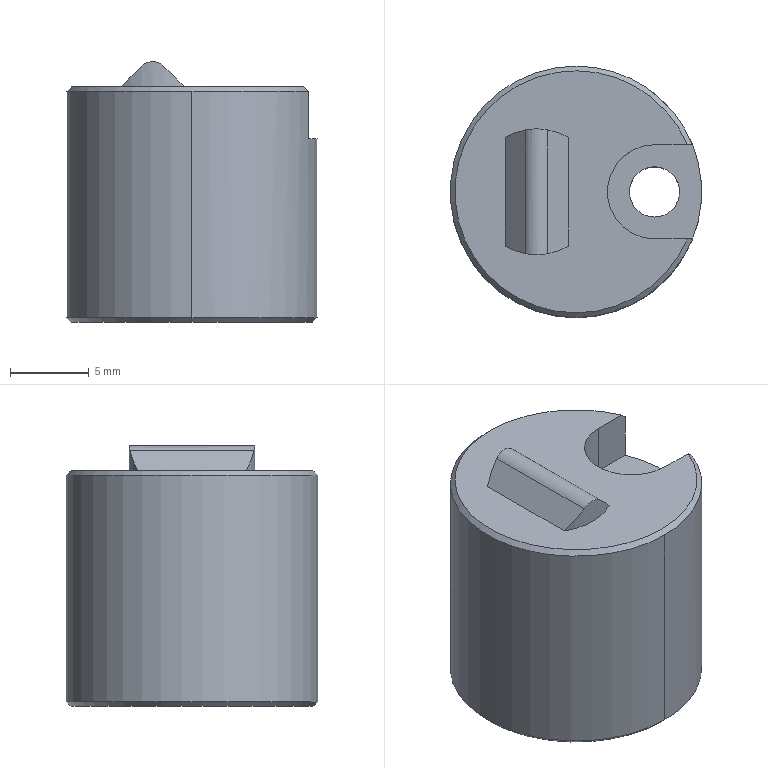Part | Creo | 1 solid | 18 faces | box 16 x 16 x 16.6 mm | volume 2845 mm3 | cylinder 8 | plane 7 | cone 3 | commonest cylinder face diameters 3.2 x2 8 x2 16 x2 2 x1 6 x1
STEP:
#1=CARTESIAN_POINT('',(0.,0.,0.));
#2=DIRECTION('',(0.,0.,1.));
#3=DIRECTION('',(1.,0.,0.));
#4=AXIS2_PLACEMENT_3D('',#1,#2,#3);
#5=CARTESIAN_POINT('',(-123.408,-41.65,-27.828));
#6=VERTEX_POINT('',#5);
#7=CARTESIAN_POINT('',(-130.5,-52.35,-27.828));
#8=VERTEX_POINT('',#7);
#9=CARTESIAN_POINT('',(-130.5,-44.65,-27.828));
#10=DIRECTION('',(0.,0.,1.));
#11=DIRECTION('',(0.921,0.3896,0.));
#12=AXIS2_PLACEMENT_3D('',#9,#10,#11);
#13=CIRCLE('',#12,7.7);
#14=EDGE_CURVE('',#6,#8,#13,.T.);
#15=ORIENTED_EDGE('',*,*,#14,.F.);
#16=CARTESIAN_POINT('',(-125.5,-41.65,-27.828));
#17=VERTEX_POINT('',#16);
#18=CARTESIAN_POINT('',(-125.5,-41.65,-27.828));
#19=DIRECTION('',(1.,0.,0.));
#20=VECTOR('',#19,2.092);
#21=LINE('',#18,#20);
#22=EDGE_CURVE('',#17,#6,#21,.T.);
#23=ORIENTED_EDGE('',*,*,#22,.F.);
#24=CARTESIAN_POINT('',(-125.5,-47.65,-27.828));
#25=VERTEX_POINT('',#24);
#26=CARTESIAN_POINT('',(-125.5,-44.65,-27.828));
#27=DIRECTION('',(0.,0.,-1.));
#28=DIRECTION('',(0.,-1.,0.));
#29=AXIS2_PLACEMENT_3D('',#26,#27,#28);
#30=CIRCLE('',#29,3.);
#31=EDGE_CURVE('',#25,#17,#30,.T.);
#32=ORIENTED_EDGE('',*,*,#31,.F.);
#33=CARTESIAN_POINT('',(-123.408,-47.65,-27.828));
#34=VERTEX_POINT('',#33);
#35=CARTESIAN_POINT('',(-123.408,-47.65,-27.828));
#36=DIRECTION('',(-1.,0.,0.));
#37=VECTOR('',#36,2.092);
#38=LINE('',#35,#37);
#39=EDGE_CURVE('',#34,#25,#38,.T.);
#40=ORIENTED_EDGE('',*,*,#39,.F.);
#41=CARTESIAN_POINT('',(-130.5,-44.65,-27.828));
#42=DIRECTION('',(0.,0.,1.));
#43=DIRECTION('',(0.,-1.,0.));
#44=AXIS2_PLACEMENT_3D('',#41,#42,#43);
#45=CIRCLE('',#44,7.7);
#46=EDGE_CURVE('',#8,#34,#45,.T.);
#47=ORIENTED_EDGE('',*,*,#46,.F.);
#48=EDGE_LOOP('',(#15,#23,#32,#40,#47));
#49=FACE_OUTER_BOUND('',#48,.F.);
#50=CARTESIAN_POINT('',(-135.014,-41.194,-27.828));
#51=VERTEX_POINT('',#50);
#52=CARTESIAN_POINT('',(-133.,-40.65,-27.828));
#53=VERTEX_POINT('',#52);
#54=CARTESIAN_POINT('',(-133.,-44.65,-27.828));
#55=DIRECTION('',(0.,0.,-1.));
#56=DIRECTION('',(-0.5036,0.864,0.));
#57=AXIS2_PLACEMENT_3D('',#54,#55,#56);
#58=CIRCLE('',#57,4.);
#59=EDGE_CURVE('',#51,#53,#58,.T.);
#60=ORIENTED_EDGE('',*,*,#59,.F.);
#61=CARTESIAN_POINT('',(-135.014,-48.106,-27.828));
#62=VERTEX_POINT('',#61);
#63=CARTESIAN_POINT('',(-135.014,-48.106,-27.828));
#64=DIRECTION('',(0.,1.,0.));
#65=VECTOR('',#64,6.912);
#66=LINE('',#63,#65);
#67=EDGE_CURVE('',#62,#51,#66,.T.);
#68=ORIENTED_EDGE('',*,*,#67,.F.);
#69=CARTESIAN_POINT('',(-133.,-48.65,-27.828));
#70=VERTEX_POINT('',#69);
#71=CARTESIAN_POINT('',(-133.,-44.65,-27.828));
#72=DIRECTION('',(0.,0.,-1.));
#73=DIRECTION('',(0.,-1.,0.));
#74=AXIS2_PLACEMENT_3D('',#71,#72,#73);
#75=CIRCLE('',#74,4.);
#76=EDGE_CURVE('',#70,#62,#75,.T.);
#77=ORIENTED_EDGE('',*,*,#76,.F.);
#78=CARTESIAN_POINT('',(-130.986,-48.106,-27.828));
#79=VERTEX_POINT('',#78);
#80=CARTESIAN_POINT('',(-133.,-44.65,-27.828));
#81=DIRECTION('',(0.,0.,-1.));
#82=DIRECTION('',(0.5036,-0.864,0.));
#83=AXIS2_PLACEMENT_3D('',#80,#81,#82);
#84=CIRCLE('',#83,4.);
#85=EDGE_CURVE('',#79,#70,#84,.T.);
#86=ORIENTED_EDGE('',*,*,#85,.F.);
#87=CARTESIAN_POINT('',(-130.986,-41.194,-27.828));
#88=VERTEX_POINT('',#87);
#89=CARTESIAN_POINT('',(-130.986,-48.106,-27.828));
#90=DIRECTION('',(0.,1.,0.));
#91=VECTOR('',#90,6.912);
#92=LINE('',#89,#91);
#93=EDGE_CURVE('',#79,#88,#92,.T.);
#94=ORIENTED_EDGE('',*,*,#93,.T.);
#95=CARTESIAN_POINT('',(-133.,-44.65,-27.828));
#96=DIRECTION('',(0.,0.,-1.));
#97=DIRECTION('',(0.,1.,0.));
#98=AXIS2_PLACEMENT_3D('',#95,#96,#97);
#99=CIRCLE('',#98,4.);
#100=EDGE_CURVE('',#53,#88,#99,.T.);
#101=ORIENTED_EDGE('',*,*,#100,.F.);
#102=EDGE_LOOP('',(#60,#68,#77,#86,#94,#101));
#103=FACE_BOUND('',#102,.F.);
#104=CARTESIAN_POINT('',(-130.5,-44.65,-27.828));
#105=DIRECTION('',(0.,0.,1.));
#106=DIRECTION('',(0.,1.,0.));
#107=AXIS2_PLACEMENT_3D('',#104,#105,#106);
#108=PLANE('',#107);
#109=ADVANCED_FACE('',(#49,#103),#108,.T.);
#110=CARTESIAN_POINT('',(-132.293,-40.713,-26.52));
#111=VERTEX_POINT('',#110);
#112=CARTESIAN_POINT('',(-131.842,-40.794,-26.971));
#113=CARTESIAN_POINT('',(-131.406,-40.949,-27.408));
#114=CARTESIAN_POINT('',(-130.986,-41.194,-27.828));
#115=B_SPLINE_CURVE_WITH_KNOTS('',3,(#110,#112,#113,#114),.UNSPECIFIED.,.F.,.F.,(4,4),(0.,1.),.UNSPECIFIED.);
#116=EDGE_CURVE('',#111,#88,#115,.T.);
#117=ORIENTED_EDGE('',*,*,#116,.F.);
#118=CARTESIAN_POINT('',(-133.707,-40.713,-26.52));
#119=VERTEX_POINT('',#118);
#120=CARTESIAN_POINT('',(-133.707,-40.713,-26.52));
#121=CARTESIAN_POINT('',(-133.652,-40.703,-26.466));
#122=CARTESIAN_POINT('',(-133.534,-40.684,-26.372));
#123=CARTESIAN_POINT('',(-133.33,-40.662,-26.275));
#124=CARTESIAN_POINT('',(-133.112,-40.65,-26.226));
#125=CARTESIAN_POINT('',(-132.889,-40.649,-26.225));
#126=CARTESIAN_POINT('',(-132.67,-40.662,-26.275));
#127=CARTESIAN_POINT('',(-132.466,-40.684,-26.372));
#128=CARTESIAN_POINT('',(-132.348,-40.703,-26.466));
#129=CARTESIAN_POINT('',(-132.293,-40.713,-26.52));
#130=B_SPLINE_CURVE_WITH_KNOTS('',3,(#120,#121,#122,#123,#124,#125,#126,#127,#128,#129),.UNSPECIFIED.,.F.,.F.,(4,1,1,1,1,1,1,4),(0.,0.1429,0.2857,0.4286,0.5714,0.7143,0.8571,1.),.UNSPECIFIED.);
#131=EDGE_CURVE('',#119,#111,#130,.T.);
#132=ORIENTED_EDGE('',*,*,#131,.F.);
#133=CARTESIAN_POINT('',(-135.014,-41.194,-27.828));
#134=CARTESIAN_POINT('',(-134.594,-40.949,-27.408));
#135=CARTESIAN_POINT('',(-134.158,-40.794,-26.971));
#136=CARTESIAN_POINT('',(-133.707,-40.713,-26.52));
#137=B_SPLINE_CURVE_WITH_KNOTS('',3,(#133,#134,#135,#136),.UNSPECIFIED.,.F.,.F.,(4,4),(0.,1.),.UNSPECIFIED.);
#138=EDGE_CURVE('',#51,#119,#137,.T.);
#139=ORIENTED_EDGE('',*,*,#138,.F.);
#140=ORIENTED_EDGE('',*,*,#59,.T.);
#141=ORIENTED_EDGE('',*,*,#100,.T.);
#142=EDGE_LOOP('',(#117,#132,#139,#140,#141));
#143=FACE_OUTER_BOUND('',#142,.F.);
#144=CARTESIAN_POINT('',(-133.,-44.65,-11.828));
#145=DIRECTION('',(0.,0.,-1.));
#146=DIRECTION('',(0.,-1.,0.));
#147=AXIS2_PLACEMENT_3D('',#144,#145,#146);
#148=CYLINDRICAL_SURFACE('',#147,4.);
#149=ADVANCED_FACE('',(#143),#148,.T.);
#150=ORIENTED_EDGE('',*,*,#93,.F.);
#151=CARTESIAN_POINT('',(-132.293,-48.587,-26.52));
#152=VERTEX_POINT('',#151);
#153=CARTESIAN_POINT('',(-130.986,-48.106,-27.828));
#154=CARTESIAN_POINT('',(-131.406,-48.351,-27.408));
#155=CARTESIAN_POINT('',(-131.842,-48.506,-26.971));
#156=CARTESIAN_POINT('',(-132.293,-48.587,-26.52));
#157=B_SPLINE_CURVE_WITH_KNOTS('',3,(#153,#154,#155,#156),.UNSPECIFIED.,.F.,.F.,(4,4),(0.,1.),.UNSPECIFIED.);
#158=EDGE_CURVE('',#79,#152,#157,.T.);
#159=ORIENTED_EDGE('',*,*,#158,.T.);
#160=CARTESIAN_POINT('',(-132.293,-48.587,-26.52));
#161=DIRECTION('',(0.,1.,0.));
#162=VECTOR('',#161,7.874);
#163=LINE('',#160,#162);
#164=EDGE_CURVE('',#152,#111,#163,.T.);
#165=ORIENTED_EDGE('',*,*,#164,.T.);
#166=ORIENTED_EDGE('',*,*,#116,.T.);
#167=EDGE_LOOP('',(#150,#159,#165,#166));
#168=FACE_OUTER_BOUND('',#167,.F.);
#169=CARTESIAN_POINT('',(-132.293,-40.65,-26.52));
#170=DIRECTION('',(-0.7071,0.,-0.7071));
#171=DIRECTION('',(-0.7071,0.,0.7071));
#172=AXIS2_PLACEMENT_3D('',#169,#170,#171);
#173=PLANE('',#172);
#174=ADVANCED_FACE('',(#168),#173,.F.);
#175=CARTESIAN_POINT('',(-133.707,-48.587,-26.52));
#176=VERTEX_POINT('',#175);
#177=CARTESIAN_POINT('',(-134.158,-48.506,-26.971));
#178=CARTESIAN_POINT('',(-134.594,-48.351,-27.408));
#179=CARTESIAN_POINT('',(-135.014,-48.106,-27.828));
#180=B_SPLINE_CURVE_WITH_KNOTS('',3,(#175,#177,#178,#179),.UNSPECIFIED.,.F.,.F.,(4,4),(0.,1.),.UNSPECIFIED.);
#181=EDGE_CURVE('',#176,#62,#180,.T.);
#182=ORIENTED_EDGE('',*,*,#181,.F.);
#183=CARTESIAN_POINT('',(-133.,-48.65,-26.228));
#184=VERTEX_POINT('',#183);
#185=CARTESIAN_POINT('',(-133.065,-48.65,-26.228));
#186=CARTESIAN_POINT('',(-133.194,-48.647,-26.24));
#187=CARTESIAN_POINT('',(-133.383,-48.633,-26.296));
#188=CARTESIAN_POINT('',(-133.558,-48.612,-26.39));
#189=CARTESIAN_POINT('',(-133.66,-48.596,-26.473));
#190=CARTESIAN_POINT('',(-133.707,-48.587,-26.52));
#191=B_SPLINE_CURVE_WITH_KNOTS('',3,(#183,#185,#186,#187,#188,#189,#190),.UNSPECIFIED.,.F.,.F.,(4,1,1,1,4),(0.,0.25,0.5,0.75,1.),.UNSPECIFIED.);
#192=EDGE_CURVE('',#184,#176,#191,.T.);
#193=ORIENTED_EDGE('',*,*,#192,.F.);
#194=CARTESIAN_POINT('',(-132.293,-48.587,-26.52));
#195=CARTESIAN_POINT('',(-132.34,-48.595,-26.473));
#196=CARTESIAN_POINT('',(-132.442,-48.612,-26.39));
#197=CARTESIAN_POINT('',(-132.617,-48.633,-26.297));
#198=CARTESIAN_POINT('',(-132.806,-48.647,-26.24));
#199=CARTESIAN_POINT('',(-132.934,-48.65,-26.228));
#200=CARTESIAN_POINT('',(-133.,-48.65,-26.228));
#201=B_SPLINE_CURVE_WITH_KNOTS('',3,(#194,#195,#196,#197,#198,#199,#200),.UNSPECIFIED.,.F.,.F.,(4,1,1,1,4),(0.,0.25,0.5,0.75,1.),.UNSPECIFIED.);
#202=EDGE_CURVE('',#152,#184,#201,.T.);
#203=ORIENTED_EDGE('',*,*,#202,.F.);
#204=ORIENTED_EDGE('',*,*,#158,.F.);
#205=ORIENTED_EDGE('',*,*,#85,.T.);
#206=ORIENTED_EDGE('',*,*,#76,.T.);
#207=EDGE_LOOP('',(#182,#193,#203,#204,#205,#206));
#208=FACE_OUTER_BOUND('',#207,.F.);
#209=CARTESIAN_POINT('',(-133.,-44.65,-11.828));
#210=DIRECTION('',(0.,0.,-1.));
#211=DIRECTION('',(0.,-1.,0.));
#212=AXIS2_PLACEMENT_3D('',#209,#210,#211);
#213=CYLINDRICAL_SURFACE('',#212,4.);
#214=ADVANCED_FACE('',(#208),#213,.T.);
#215=ORIENTED_EDGE('',*,*,#67,.T.);
#216=ORIENTED_EDGE('',*,*,#138,.T.);
#217=CARTESIAN_POINT('',(-133.707,-40.713,-26.52));
#218=DIRECTION('',(0.,-1.,0.));
#219=VECTOR('',#218,7.874);
#220=LINE('',#217,#219);
#221=EDGE_CURVE('',#119,#176,#220,.T.);
#222=ORIENTED_EDGE('',*,*,#221,.T.);
#223=ORIENTED_EDGE('',*,*,#181,.T.);
#224=EDGE_LOOP('',(#215,#216,#222,#223));
#225=FACE_OUTER_BOUND('',#224,.F.);
#226=CARTESIAN_POINT('',(-135.014,-40.65,-27.828));
#227=DIRECTION('',(0.7071,0.,-0.7071));
#228=DIRECTION('',(-0.7071,0.,-0.7071));
#229=AXIS2_PLACEMENT_3D('',#226,#227,#228);
#230=PLANE('',#229);
#231=ADVANCED_FACE('',(#225),#230,.F.);
#232=ORIENTED_EDGE('',*,*,#221,.F.);
#233=ORIENTED_EDGE('',*,*,#131,.T.);
#234=ORIENTED_EDGE('',*,*,#164,.F.);
#235=ORIENTED_EDGE('',*,*,#202,.T.);
#236=ORIENTED_EDGE('',*,*,#192,.T.);
#237=EDGE_LOOP('',(#232,#233,#234,#235,#236));
#238=FACE_OUTER_BOUND('',#237,.F.);
#239=CARTESIAN_POINT('',(-133.,-40.65,-27.227));
#240=DIRECTION('',(0.,-1.,0.));
#241=DIRECTION('',(0.,0.,1.));
#242=AXIS2_PLACEMENT_3D('',#239,#240,#241);
#243=CYLINDRICAL_SURFACE('',#242,1.);
#244=ADVANCED_FACE('',(#238),#243,.T.);
#245=CARTESIAN_POINT('',(-130.5,-36.65,-28.128));
#246=VERTEX_POINT('',#245);
#247=CARTESIAN_POINT('',(-130.5,-52.65,-28.128));
#248=VERTEX_POINT('',#247);
#249=CARTESIAN_POINT('',(-130.5,-44.65,-28.128));
#250=DIRECTION('',(0.,0.,1.));
#251=DIRECTION('',(0.,1.,0.));
#252=AXIS2_PLACEMENT_3D('',#249,#250,#251);
#253=CIRCLE('',#252,8.);
#254=EDGE_CURVE('',#246,#248,#253,.T.);
#255=ORIENTED_EDGE('',*,*,#254,.F.);
#256=CARTESIAN_POINT('',(-123.084,-41.65,-28.128));
#257=VERTEX_POINT('',#256);
#258=CARTESIAN_POINT('',(-130.5,-44.65,-28.128));
#259=DIRECTION('',(0.,0.,1.));
#260=DIRECTION('',(0.927,0.375,0.));
#261=AXIS2_PLACEMENT_3D('',#258,#259,#260);
#262=CIRCLE('',#261,8.);
#263=EDGE_CURVE('',#257,#246,#262,.T.);
#264=ORIENTED_EDGE('',*,*,#263,.F.);
#265=CARTESIAN_POINT('',(-123.408,-41.65,-27.828));
#266=CARTESIAN_POINT('',(-123.373,-41.65,-27.86));
#267=CARTESIAN_POINT('',(-123.301,-41.65,-27.927));
#268=CARTESIAN_POINT('',(-123.193,-41.65,-28.027));
#269=CARTESIAN_POINT('',(-123.12,-41.65,-28.094));
#270=B_SPLINE_CURVE_WITH_KNOTS('',3,(#265,#266,#267,#268,#269,#256),.UNSPECIFIED.,.F.,.F.,(4,1,1,4),(0.,0.3333,0.6667,1.),.UNSPECIFIED.);
#271=EDGE_CURVE('',#6,#257,#270,.T.);
#272=ORIENTED_EDGE('',*,*,#271,.F.);
#273=ORIENTED_EDGE('',*,*,#14,.T.);
#274=ORIENTED_EDGE('',*,*,#46,.T.);
#275=CARTESIAN_POINT('',(-123.084,-47.65,-28.128));
#276=VERTEX_POINT('',#275);
#277=CARTESIAN_POINT('',(-123.12,-47.65,-28.094));
#278=CARTESIAN_POINT('',(-123.193,-47.65,-28.027));
#279=CARTESIAN_POINT('',(-123.301,-47.65,-27.927));
#280=CARTESIAN_POINT('',(-123.373,-47.65,-27.86));
#281=CARTESIAN_POINT('',(-123.408,-47.65,-27.828));
#282=B_SPLINE_CURVE_WITH_KNOTS('',3,(#275,#277,#278,#279,#280,#281),.UNSPECIFIED.,.F.,.F.,(4,1,1,4),(0.,0.3333,0.6667,1.),.UNSPECIFIED.);
#283=EDGE_CURVE('',#276,#34,#282,.T.);
#284=ORIENTED_EDGE('',*,*,#283,.F.);
#285=CARTESIAN_POINT('',(-130.5,-44.65,-28.128));
#286=DIRECTION('',(0.,0.,1.));
#287=DIRECTION('',(0.,-1.,0.));
#288=AXIS2_PLACEMENT_3D('',#285,#286,#287);
#289=CIRCLE('',#288,8.);
#290=EDGE_CURVE('',#248,#276,#289,.T.);
#291=ORIENTED_EDGE('',*,*,#290,.F.);
#292=EDGE_LOOP('',(#255,#264,#272,#273,#274,#284,#291));
#293=FACE_OUTER_BOUND('',#292,.F.);
#294=CARTESIAN_POINT('',(-130.5,-44.65,-27.977));
#295=DIRECTION('',(0.,0.,-1.));
#296=DIRECTION('',(0.,-1.,0.));
#297=AXIS2_PLACEMENT_3D('',#294,#295,#296);
#298=CONICAL_SURFACE('',#297,7.85,45.);
#299=ADVANCED_FACE('',(#293),#298,.T.);
#300=ORIENTED_EDGE('',*,*,#254,.T.);
#301=CARTESIAN_POINT('',(-130.5,-52.65,-42.528));
#302=VERTEX_POINT('',#301);
#303=CARTESIAN_POINT('',(-130.5,-52.65,-42.528));
#304=DIRECTION('',(0.,0.,1.));
#305=VECTOR('',#304,14.4);
#306=LINE('',#303,#305);
#307=EDGE_CURVE('',#302,#248,#306,.T.);
#308=ORIENTED_EDGE('',*,*,#307,.F.);
#309=CARTESIAN_POINT('',(-130.5,-36.65,-42.528));
#310=VERTEX_POINT('',#309);
#311=CARTESIAN_POINT('',(-130.5,-44.65,-42.528));
#312=DIRECTION('',(0.,0.,-1.));
#313=DIRECTION('',(0.,-1.,0.));
#314=AXIS2_PLACEMENT_3D('',#311,#312,#313);
#315=CIRCLE('',#314,8.);
#316=EDGE_CURVE('',#302,#310,#315,.T.);
#317=ORIENTED_EDGE('',*,*,#316,.T.);
#318=CARTESIAN_POINT('',(-130.5,-36.65,-42.528));
#319=DIRECTION('',(0.,0.,1.));
#320=VECTOR('',#319,14.4);
#321=LINE('',#318,#320);
#322=EDGE_CURVE('',#310,#246,#321,.T.);
#323=ORIENTED_EDGE('',*,*,#322,.T.);
#324=EDGE_LOOP('',(#300,#308,#317,#323));
#325=FACE_OUTER_BOUND('',#324,.F.);
#326=CARTESIAN_POINT('',(-130.5,-44.65,-42.828));
#327=DIRECTION('',(0.,0.,1.));
#328=DIRECTION('',(0.,1.,0.));
#329=AXIS2_PLACEMENT_3D('',#326,#327,#328);
#330=CYLINDRICAL_SURFACE('',#329,8.);
#331=ADVANCED_FACE('',(#325),#330,.T.);
#332=CARTESIAN_POINT('',(-123.084,-47.65,-31.128));
#333=VERTEX_POINT('',#332);
#334=CARTESIAN_POINT('',(-123.084,-47.65,-31.128));
#335=DIRECTION('',(0.,0.,1.));
#336=VECTOR('',#335,3.);
#337=LINE('',#334,#336);
#338=EDGE_CURVE('',#333,#276,#337,.T.);
#339=ORIENTED_EDGE('',*,*,#338,.F.);
#340=CARTESIAN_POINT('',(-123.084,-41.65,-31.128));
#341=VERTEX_POINT('',#340);
#342=CARTESIAN_POINT('',(-130.5,-44.65,-31.128));
#343=DIRECTION('',(0.,0.,1.));
#344=DIRECTION('',(0.927,-0.375,0.));
#345=AXIS2_PLACEMENT_3D('',#342,#343,#344);
#346=CIRCLE('',#345,8.);
#347=EDGE_CURVE('',#333,#341,#346,.T.);
#348=ORIENTED_EDGE('',*,*,#347,.T.);
#349=CARTESIAN_POINT('',(-123.084,-41.65,-28.128));
#350=DIRECTION('',(0.,0.,-1.));
#351=VECTOR('',#350,3.);
#352=LINE('',#349,#351);
#353=EDGE_CURVE('',#257,#341,#352,.T.);
#354=ORIENTED_EDGE('',*,*,#353,.F.);
#355=ORIENTED_EDGE('',*,*,#263,.T.);
#356=ORIENTED_EDGE('',*,*,#322,.F.);
#357=CARTESIAN_POINT('',(-130.5,-44.65,-42.528));
#358=DIRECTION('',(0.,0.,-1.));
#359=DIRECTION('',(0.,1.,0.));
#360=AXIS2_PLACEMENT_3D('',#357,#358,#359);
#361=CIRCLE('',#360,8.);
#362=EDGE_CURVE('',#310,#302,#361,.T.);
#363=ORIENTED_EDGE('',*,*,#362,.T.);
#364=ORIENTED_EDGE('',*,*,#307,.T.);
#365=ORIENTED_EDGE('',*,*,#290,.T.);
#366=EDGE_LOOP('',(#339,#348,#354,#355,#356,#363,#364,#365));
#367=FACE_OUTER_BOUND('',#366,.F.);
#368=CARTESIAN_POINT('',(-130.5,-44.65,-42.828));
#369=DIRECTION('',(0.,0.,1.));
#370=DIRECTION('',(0.,1.,0.));
#371=AXIS2_PLACEMENT_3D('',#368,#369,#370);
#372=CYLINDRICAL_SURFACE('',#371,8.);
#373=ADVANCED_FACE('',(#367),#372,.T.);
#374=ORIENTED_EDGE('',*,*,#338,.T.);
#375=ORIENTED_EDGE('',*,*,#283,.T.);
#376=ORIENTED_EDGE('',*,*,#39,.T.);
#377=CARTESIAN_POINT('',(-125.5,-47.65,-31.128));
#378=VERTEX_POINT('',#377);
#379=CARTESIAN_POINT('',(-125.5,-47.65,-27.828));
#380=DIRECTION('',(0.,0.,-1.));
#381=VECTOR('',#380,3.3);
#382=LINE('',#379,#381);
#383=EDGE_CURVE('',#25,#378,#382,.T.);
#384=ORIENTED_EDGE('',*,*,#383,.T.);
#385=CARTESIAN_POINT('',(-125.5,-47.65,-31.128));
#386=DIRECTION('',(1.,0.,0.));
#387=VECTOR('',#386,2.416);
#388=LINE('',#385,#387);
#389=EDGE_CURVE('',#378,#333,#388,.T.);
#390=ORIENTED_EDGE('',*,*,#389,.T.);
#391=EDGE_LOOP('',(#374,#375,#376,#384,#390));
#392=FACE_OUTER_BOUND('',#391,.F.);
#393=CARTESIAN_POINT('',(-125.5,-47.65,-31.128));
#394=DIRECTION('',(0.,-1.,0.));
#395=DIRECTION('',(1.,0.,0.));
#396=AXIS2_PLACEMENT_3D('',#393,#394,#395);
#397=PLANE('',#396);
#398=ADVANCED_FACE('',(#392),#397,.F.);
#399=ORIENTED_EDGE('',*,*,#31,.T.);
#400=CARTESIAN_POINT('',(-125.5,-41.65,-31.128));
#401=VERTEX_POINT('',#400);
#402=CARTESIAN_POINT('',(-125.5,-41.65,-31.128));
#403=DIRECTION('',(0.,0.,1.));
#404=VECTOR('',#403,3.3);
#405=LINE('',#402,#404);
#406=EDGE_CURVE('',#401,#17,#405,.T.);
#407=ORIENTED_EDGE('',*,*,#406,.F.);
#408=CARTESIAN_POINT('',(-125.5,-44.65,-31.128));
#409=DIRECTION('',(0.,0.,1.));
#410=DIRECTION('',(0.,1.,0.));
#411=AXIS2_PLACEMENT_3D('',#408,#409,#410);
#412=CIRCLE('',#411,3.);
#413=EDGE_CURVE('',#401,#378,#412,.T.);
#414=ORIENTED_EDGE('',*,*,#413,.T.);
#415=ORIENTED_EDGE('',*,*,#383,.F.);
#416=EDGE_LOOP('',(#399,#407,#414,#415));
#417=FACE_OUTER_BOUND('',#416,.F.);
#418=CARTESIAN_POINT('',(-125.5,-44.65,-27.828));
#419=DIRECTION('',(0.,0.,-1.));
#420=DIRECTION('',(0.,-1.,0.));
#421=AXIS2_PLACEMENT_3D('',#418,#419,#420);
#422=CYLINDRICAL_SURFACE('',#421,3.);
#423=ADVANCED_FACE('',(#417),#422,.F.);
#424=ORIENTED_EDGE('',*,*,#353,.T.);
#425=CARTESIAN_POINT('',(-123.084,-41.65,-31.128));
#426=DIRECTION('',(-1.,0.,0.));
#427=VECTOR('',#426,2.416);
#428=LINE('',#425,#427);
#429=EDGE_CURVE('',#341,#401,#428,.T.);
#430=ORIENTED_EDGE('',*,*,#429,.T.);
#431=ORIENTED_EDGE('',*,*,#406,.T.);
#432=ORIENTED_EDGE('',*,*,#22,.T.);
#433=ORIENTED_EDGE('',*,*,#271,.T.);
#434=EDGE_LOOP('',(#424,#430,#431,#432,#433));
#435=FACE_OUTER_BOUND('',#434,.F.);
#436=CARTESIAN_POINT('',(-119.5,-41.65,-31.128));
#437=DIRECTION('',(0.,1.,0.));
#438=DIRECTION('',(-1.,0.,0.));
#439=AXIS2_PLACEMENT_3D('',#436,#437,#438);
#440=PLANE('',#439);
#441=ADVANCED_FACE('',(#435),#440,.F.);
#442=ORIENTED_EDGE('',*,*,#389,.F.);
#443=ORIENTED_EDGE('',*,*,#413,.F.);
#444=ORIENTED_EDGE('',*,*,#429,.F.);
#445=ORIENTED_EDGE('',*,*,#347,.F.);
#446=EDGE_LOOP('',(#442,#443,#444,#445));
#447=FACE_OUTER_BOUND('',#446,.F.);
#448=CARTESIAN_POINT('',(-125.5,-46.25,-31.128));
#449=VERTEX_POINT('',#448);
#450=CARTESIAN_POINT('',(-125.5,-43.05,-31.128));
#451=VERTEX_POINT('',#450);
#452=CARTESIAN_POINT('',(-125.5,-44.65,-31.128));
#453=DIRECTION('',(0.,0.,-1.));
#454=DIRECTION('',(0.,-1.,0.));
#455=AXIS2_PLACEMENT_3D('',#452,#453,#454);
#456=CIRCLE('',#455,1.6);
#457=EDGE_CURVE('',#449,#451,#456,.T.);
#458=ORIENTED_EDGE('',*,*,#457,.F.);
#459=CARTESIAN_POINT('',(-125.5,-44.65,-31.128));
#460=DIRECTION('',(0.,0.,-1.));
#461=DIRECTION('',(0.,1.,0.));
#462=AXIS2_PLACEMENT_3D('',#459,#460,#461);
#463=CIRCLE('',#462,1.6);
#464=EDGE_CURVE('',#451,#449,#463,.T.);
#465=ORIENTED_EDGE('',*,*,#464,.F.);
#466=EDGE_LOOP('',(#458,#465));
#467=FACE_BOUND('',#466,.F.);
#468=CARTESIAN_POINT('',(-130.5,-44.65,-31.128));
#469=DIRECTION('',(0.,0.,1.));
#470=DIRECTION('',(0.,1.,0.));
#471=AXIS2_PLACEMENT_3D('',#468,#469,#470);
#472=PLANE('',#471);
#473=ADVANCED_FACE('',(#447,#467),#472,.T.);
#474=ORIENTED_EDGE('',*,*,#457,.T.);
#475=CARTESIAN_POINT('',(-125.5,-43.05,-42.828));
#476=VERTEX_POINT('',#475);
#477=CARTESIAN_POINT('',(-125.5,-43.05,-31.128));
#478=DIRECTION('',(0.,0.,-1.));
#479=VECTOR('',#478,11.7);
#480=LINE('',#477,#479);
#481=EDGE_CURVE('',#451,#476,#480,.T.);
#482=ORIENTED_EDGE('',*,*,#481,.T.);
#483=CARTESIAN_POINT('',(-125.5,-46.25,-42.828));
#484=VERTEX_POINT('',#483);
#485=CARTESIAN_POINT('',(-125.5,-44.65,-42.828));
#486=DIRECTION('',(0.,0.,1.));
#487=DIRECTION('',(0.,1.,0.));
#488=AXIS2_PLACEMENT_3D('',#485,#486,#487);
#489=CIRCLE('',#488,1.6);
#490=EDGE_CURVE('',#476,#484,#489,.T.);
#491=ORIENTED_EDGE('',*,*,#490,.T.);
#492=CARTESIAN_POINT('',(-125.5,-46.25,-31.128));
#493=DIRECTION('',(0.,0.,-1.));
#494=VECTOR('',#493,11.7);
#495=LINE('',#492,#494);
#496=EDGE_CURVE('',#449,#484,#495,.T.);
#497=ORIENTED_EDGE('',*,*,#496,.F.);
#498=EDGE_LOOP('',(#474,#482,#491,#497));
#499=FACE_OUTER_BOUND('',#498,.F.);
#500=CARTESIAN_POINT('',(-125.5,-44.65,-27.828));
#501=DIRECTION('',(0.,0.,-1.));
#502=DIRECTION('',(0.,-1.,0.));
#503=AXIS2_PLACEMENT_3D('',#500,#501,#502);
#504=CYLINDRICAL_SURFACE('',#503,1.6);
#505=ADVANCED_FACE('',(#499),#504,.F.);
#506=ORIENTED_EDGE('',*,*,#464,.T.);
#507=ORIENTED_EDGE('',*,*,#496,.T.);
#508=CARTESIAN_POINT('',(-125.5,-44.65,-42.828));
#509=DIRECTION('',(0.,0.,1.));
#510=DIRECTION('',(0.,-1.,0.));
#511=AXIS2_PLACEMENT_3D('',#508,#509,#510);
#512=CIRCLE('',#511,1.6);
#513=EDGE_CURVE('',#484,#476,#512,.T.);
#514=ORIENTED_EDGE('',*,*,#513,.T.);
#515=ORIENTED_EDGE('',*,*,#481,.F.);
#516=EDGE_LOOP('',(#506,#507,#514,#515));
#517=FACE_OUTER_BOUND('',#516,.F.);
#518=CARTESIAN_POINT('',(-125.5,-44.65,-27.828));
#519=DIRECTION('',(0.,0.,-1.));
#520=DIRECTION('',(0.,-1.,0.));
#521=AXIS2_PLACEMENT_3D('',#518,#519,#520);
#522=CYLINDRICAL_SURFACE('',#521,1.6);
#523=ADVANCED_FACE('',(#517),#522,.F.);
#524=CARTESIAN_POINT('',(-130.5,-36.95,-42.828));
#525=VERTEX_POINT('',#524);
#526=CARTESIAN_POINT('',(-130.5,-52.35,-42.828));
#527=VERTEX_POINT('',#526);
#528=CARTESIAN_POINT('',(-130.5,-44.65,-42.828));
#529=DIRECTION('',(0.,0.,-1.));
#530=DIRECTION('',(0.,1.,0.));
#531=AXIS2_PLACEMENT_3D('',#528,#529,#530);
#532=CIRCLE('',#531,7.7);
#533=EDGE_CURVE('',#525,#527,#532,.T.);
#534=ORIENTED_EDGE('',*,*,#533,.F.);
#535=CARTESIAN_POINT('',(-130.5,-44.65,-42.828));
#536=DIRECTION('',(0.,0.,-1.));
#537=DIRECTION('',(0.,-1.,0.));
#538=AXIS2_PLACEMENT_3D('',#535,#536,#537);
#539=CIRCLE('',#538,7.7);
#540=EDGE_CURVE('',#527,#525,#539,.T.);
#541=ORIENTED_EDGE('',*,*,#540,.F.);
#542=EDGE_LOOP('',(#534,#541));
#543=FACE_OUTER_BOUND('',#542,.F.);
#544=ORIENTED_EDGE('',*,*,#513,.F.);
#545=ORIENTED_EDGE('',*,*,#490,.F.);
#546=EDGE_LOOP('',(#544,#545));
#547=FACE_BOUND('',#546,.F.);
#548=CARTESIAN_POINT('',(-130.5,-44.65,-42.828));
#549=DIRECTION('',(0.,0.,1.));
#550=DIRECTION('',(0.,1.,0.));
#551=AXIS2_PLACEMENT_3D('',#548,#549,#550);
#552=PLANE('',#551);
#553=ADVANCED_FACE('',(#543,#547),#552,.F.);
#554=ORIENTED_EDGE('',*,*,#533,.T.);
#555=CARTESIAN_POINT('',(-130.5,-52.35,-42.828));
#556=DIRECTION('',(0.,-0.7071,0.7071));
#557=VECTOR('',#556,0.4243);
#558=LINE('',#555,#557);
#559=EDGE_CURVE('',#527,#302,#558,.T.);
#560=ORIENTED_EDGE('',*,*,#559,.T.);
#561=ORIENTED_EDGE('',*,*,#362,.F.);
#562=CARTESIAN_POINT('',(-130.5,-36.95,-42.828));
#563=DIRECTION('',(0.,0.7071,0.7071));
#564=VECTOR('',#563,0.4243);
#565=LINE('',#562,#564);
#566=EDGE_CURVE('',#525,#310,#565,.T.);
#567=ORIENTED_EDGE('',*,*,#566,.F.);
#568=EDGE_LOOP('',(#554,#560,#561,#567));
#569=FACE_OUTER_BOUND('',#568,.F.);
#570=CARTESIAN_POINT('',(-130.5,-44.65,-42.678));
#571=DIRECTION('',(0.,0.,1.));
#572=DIRECTION('',(0.,1.,0.));
#573=AXIS2_PLACEMENT_3D('',#570,#571,#572);
#574=CONICAL_SURFACE('',#573,7.85,45.);
#575=ADVANCED_FACE('',(#569),#574,.T.);
#576=ORIENTED_EDGE('',*,*,#540,.T.);
#577=ORIENTED_EDGE('',*,*,#566,.T.);
#578=ORIENTED_EDGE('',*,*,#316,.F.);
#579=ORIENTED_EDGE('',*,*,#559,.F.);
#580=EDGE_LOOP('',(#576,#577,#578,#579));
#581=FACE_OUTER_BOUND('',#580,.F.);
#582=CARTESIAN_POINT('',(-130.5,-44.65,-42.678));
#583=DIRECTION('',(0.,0.,1.));
#584=DIRECTION('',(0.,1.,0.));
#585=AXIS2_PLACEMENT_3D('',#582,#583,#584);
#586=CONICAL_SURFACE('',#585,7.85,45.);
#587=ADVANCED_FACE('',(#581),#586,.T.);
#588=CLOSED_SHELL('',(#109,#149,#174,#214,#231,#244,#299,#331,#373,#398,#423,#441,#473,#505,#523,#553,#575,#587));
#589=MANIFOLD_SOLID_BREP('',#588);
#590=(LENGTH_UNIT()NAMED_UNIT(*)SI_UNIT(.MILLI.,.METRE.));
#591=UNCERTAINTY_MEASURE_WITH_UNIT(LENGTH_MEASURE(0.002806),#590,'','');
#592=(NAMED_UNIT(*)PLANE_ANGLE_UNIT()SI_UNIT($,.RADIAN.));
#593=PLANE_ANGLE_MEASURE_WITH_UNIT(PLANE_ANGLE_MEASURE(0.01745),#592);
#594=(CONVERSION_BASED_UNIT('DEGREE',#593)NAMED_UNIT(*)PLANE_ANGLE_UNIT());
#595=(NAMED_UNIT(*)SI_UNIT($,.STERADIAN.)SOLID_ANGLE_UNIT());
#596=(GEOMETRIC_REPRESENTATION_CONTEXT(3)GLOBAL_UNCERTAINTY_ASSIGNED_CONTEXT((#591))GLOBAL_UNIT_ASSIGNED_CONTEXT((#590,#594,#595))REPRESENTATION_CONTEXT('',''));
#597=ADVANCED_BREP_SHAPE_REPRESENTATION('',(#4,#589),#596);